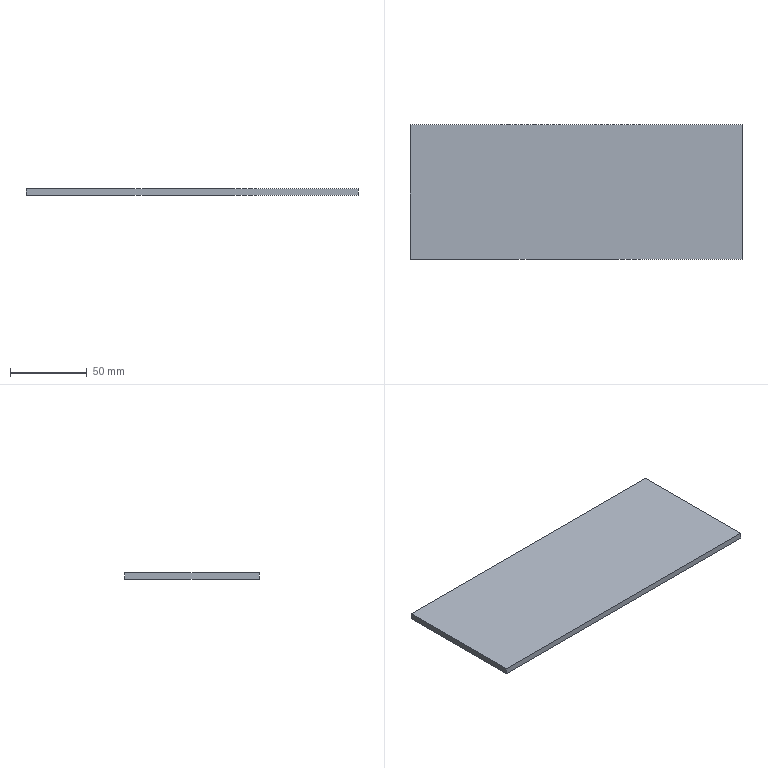Part | SolidWorks | features Extrusion 1 | 1 solid | 6 faces | box 217 x 88 x 4 mm | volume 76384 mm3 | plane 6
STEP:
#1=CARTESIAN_POINT('',(-108.5,44.,0.));
#2=VERTEX_POINT('',#1);
#3=CARTESIAN_POINT('',(-108.5,-44.,0.));
#4=VERTEX_POINT('',#3);
#5=CARTESIAN_POINT('',(-108.5,44.,0.));
#6=DIRECTION('',(0.,-1.,0.));
#7=VECTOR('',#6,1000.);
#8=LINE('',#5,#7);
#9=EDGE_CURVE('',#2,#4,#8,.T.);
#10=ORIENTED_EDGE('',*,*,#9,.T.);
#11=CARTESIAN_POINT('',(-108.5,-44.,4.));
#12=VERTEX_POINT('',#11);
#13=CARTESIAN_POINT('',(-108.5,-44.,4.));
#14=DIRECTION('',(0.,0.,-1.));
#15=VECTOR('',#14,1000.);
#16=LINE('',#13,#15);
#17=EDGE_CURVE('',#12,#4,#16,.T.);
#18=ORIENTED_EDGE('',*,*,#17,.F.);
#19=CARTESIAN_POINT('',(-108.5,44.,4.));
#20=VERTEX_POINT('',#19);
#21=CARTESIAN_POINT('',(-108.5,44.,4.));
#22=DIRECTION('',(0.,-1.,0.));
#23=VECTOR('',#22,1000.);
#24=LINE('',#21,#23);
#25=EDGE_CURVE('',#20,#12,#24,.T.);
#26=ORIENTED_EDGE('',*,*,#25,.F.);
#27=CARTESIAN_POINT('',(-108.5,44.,4.));
#28=DIRECTION('',(0.,0.,-1.));
#29=VECTOR('',#28,1000.);
#30=LINE('',#27,#29);
#31=EDGE_CURVE('',#20,#2,#30,.T.);
#32=ORIENTED_EDGE('',*,*,#31,.T.);
#33=EDGE_LOOP('',(#10,#18,#26,#32));
#34=FACE_OUTER_BOUND('',#33,.T.);
#35=CARTESIAN_POINT('',(-108.5,44.,4.));
#36=DIRECTION('',(1.,0.,0.));
#37=DIRECTION('',(0.,1.,0.));
#38=AXIS2_PLACEMENT_3D('',#35,#36,#37);
#39=PLANE('',#38);
#40=ADVANCED_FACE('',(#34),#39,.F.);
#41=CARTESIAN_POINT('',(108.5,-44.,0.));
#42=VERTEX_POINT('',#41);
#43=CARTESIAN_POINT('',(108.5,-44.,0.));
#44=DIRECTION('',(1.,0.,0.));
#45=VECTOR('',#44,1000.);
#46=LINE('',#43,#45);
#47=EDGE_CURVE('',#4,#42,#46,.T.);
#48=ORIENTED_EDGE('',*,*,#47,.T.);
#49=CARTESIAN_POINT('',(108.5,-44.,4.));
#50=VERTEX_POINT('',#49);
#51=CARTESIAN_POINT('',(108.5,-44.,4.));
#52=DIRECTION('',(0.,0.,-1.));
#53=VECTOR('',#52,1000.);
#54=LINE('',#51,#53);
#55=EDGE_CURVE('',#50,#42,#54,.T.);
#56=ORIENTED_EDGE('',*,*,#55,.F.);
#57=CARTESIAN_POINT('',(108.5,-44.,4.));
#58=DIRECTION('',(1.,0.,0.));
#59=VECTOR('',#58,1000.);
#60=LINE('',#57,#59);
#61=EDGE_CURVE('',#12,#50,#60,.T.);
#62=ORIENTED_EDGE('',*,*,#61,.F.);
#63=ORIENTED_EDGE('',*,*,#17,.T.);
#64=EDGE_LOOP('',(#48,#56,#62,#63));
#65=FACE_OUTER_BOUND('',#64,.T.);
#66=CARTESIAN_POINT('',(108.5,-44.,4.));
#67=DIRECTION('',(0.,1.,0.));
#68=DIRECTION('',(-1.,0.,0.));
#69=AXIS2_PLACEMENT_3D('',#66,#67,#68);
#70=PLANE('',#69);
#71=ADVANCED_FACE('',(#65),#70,.F.);
#72=CARTESIAN_POINT('',(108.5,44.,0.));
#73=VERTEX_POINT('',#72);
#74=CARTESIAN_POINT('',(108.5,44.,0.));
#75=DIRECTION('',(0.,1.,0.));
#76=VECTOR('',#75,1000.);
#77=LINE('',#74,#76);
#78=EDGE_CURVE('',#42,#73,#77,.T.);
#79=ORIENTED_EDGE('',*,*,#78,.T.);
#80=CARTESIAN_POINT('',(108.5,44.,4.));
#81=VERTEX_POINT('',#80);
#82=CARTESIAN_POINT('',(108.5,44.,4.));
#83=DIRECTION('',(0.,0.,-1.));
#84=VECTOR('',#83,1000.);
#85=LINE('',#82,#84);
#86=EDGE_CURVE('',#81,#73,#85,.T.);
#87=ORIENTED_EDGE('',*,*,#86,.F.);
#88=CARTESIAN_POINT('',(108.5,44.,4.));
#89=DIRECTION('',(0.,1.,0.));
#90=VECTOR('',#89,1000.);
#91=LINE('',#88,#90);
#92=EDGE_CURVE('',#50,#81,#91,.T.);
#93=ORIENTED_EDGE('',*,*,#92,.F.);
#94=ORIENTED_EDGE('',*,*,#55,.T.);
#95=EDGE_LOOP('',(#79,#87,#93,#94));
#96=FACE_OUTER_BOUND('',#95,.T.);
#97=CARTESIAN_POINT('',(108.5,44.,4.));
#98=DIRECTION('',(-1.,0.,0.));
#99=DIRECTION('',(0.,-1.,0.));
#100=AXIS2_PLACEMENT_3D('',#97,#98,#99);
#101=PLANE('',#100);
#102=ADVANCED_FACE('',(#96),#101,.F.);
#103=CARTESIAN_POINT('',(108.5,44.,0.));
#104=DIRECTION('',(-1.,0.,0.));
#105=VECTOR('',#104,1000.);
#106=LINE('',#103,#105);
#107=EDGE_CURVE('',#73,#2,#106,.T.);
#108=ORIENTED_EDGE('',*,*,#107,.T.);
#109=ORIENTED_EDGE('',*,*,#31,.F.);
#110=CARTESIAN_POINT('',(108.5,44.,4.));
#111=DIRECTION('',(-1.,0.,0.));
#112=VECTOR('',#111,1000.);
#113=LINE('',#110,#112);
#114=EDGE_CURVE('',#81,#20,#113,.T.);
#115=ORIENTED_EDGE('',*,*,#114,.F.);
#116=ORIENTED_EDGE('',*,*,#86,.T.);
#117=EDGE_LOOP('',(#108,#109,#115,#116));
#118=FACE_OUTER_BOUND('',#117,.T.);
#119=CARTESIAN_POINT('',(108.5,44.,4.));
#120=DIRECTION('',(0.,-1.,0.));
#121=DIRECTION('',(1.,0.,0.));
#122=AXIS2_PLACEMENT_3D('',#119,#120,#121);
#123=PLANE('',#122);
#124=ADVANCED_FACE('',(#118),#123,.F.);
#125=ORIENTED_EDGE('',*,*,#25,.T.);
#126=ORIENTED_EDGE('',*,*,#61,.T.);
#127=ORIENTED_EDGE('',*,*,#92,.T.);
#128=ORIENTED_EDGE('',*,*,#114,.T.);
#129=EDGE_LOOP('',(#125,#126,#127,#128));
#130=FACE_OUTER_BOUND('',#129,.T.);
#131=CARTESIAN_POINT('',(0.,0.,4.));
#132=DIRECTION('',(0.,0.,-1.));
#133=DIRECTION('',(-1.,0.,0.));
#134=AXIS2_PLACEMENT_3D('',#131,#132,#133);
#135=PLANE('',#134);
#136=ADVANCED_FACE('',(#130),#135,.F.);
#137=ORIENTED_EDGE('',*,*,#9,.F.);
#138=ORIENTED_EDGE('',*,*,#107,.F.);
#139=ORIENTED_EDGE('',*,*,#78,.F.);
#140=ORIENTED_EDGE('',*,*,#47,.F.);
#141=EDGE_LOOP('',(#137,#138,#139,#140));
#142=FACE_OUTER_BOUND('',#141,.T.);
#143=CARTESIAN_POINT('',(0.,0.,0.));
#144=DIRECTION('',(0.,0.,-1.));
#145=DIRECTION('',(-1.,0.,0.));
#146=AXIS2_PLACEMENT_3D('',#143,#144,#145);
#147=PLANE('',#146);
#148=ADVANCED_FACE('',(#142),#147,.T.);
#149=CLOSED_SHELL('',(#40,#71,#102,#124,#136,#148));
#150=MANIFOLD_SOLID_BREP('',#149);
#151=CARTESIAN_POINT('',(0.,0.,0.));
#152=DIRECTION('',(0.,0.,1.));
#153=DIRECTION('',(1.,0.,0.));
#154=AXIS2_PLACEMENT_3D('',#151,#152,#153);
#155=(LENGTH_UNIT()NAMED_UNIT(*)SI_UNIT(.MILLI.,.METRE.));
#156=UNCERTAINTY_MEASURE_WITH_UNIT(LENGTH_MEASURE(0.00001),#155,'','');
#157=(NAMED_UNIT(*)PLANE_ANGLE_UNIT()SI_UNIT($,.RADIAN.));
#158=(NAMED_UNIT(*)SI_UNIT($,.STERADIAN.)SOLID_ANGLE_UNIT());
#159=(GEOMETRIC_REPRESENTATION_CONTEXT(3)GLOBAL_UNCERTAINTY_ASSIGNED_CONTEXT((#156))GLOBAL_UNIT_ASSIGNED_CONTEXT((#155,#157,#158))REPRESENTATION_CONTEXT('',''));
#160=ADVANCED_BREP_SHAPE_REPRESENTATION('',(#150,#154),#159);